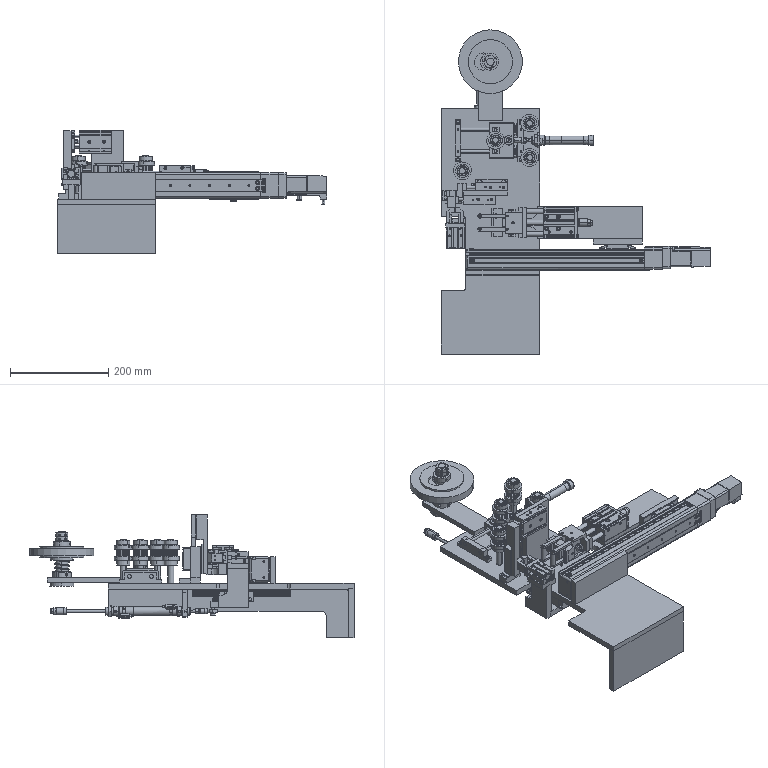Part | SolidWorks | features CompositeCurve 1 | 115 solids | 4945 faces | volume 4869772 mm3 | plane 2359 | cylinder 1769 | cone 635 | spline 156 | torus 26 | commonest cylinder face diameters 1 x140 6 x113 27 x96 24 x88 8 x82 4.134 x80